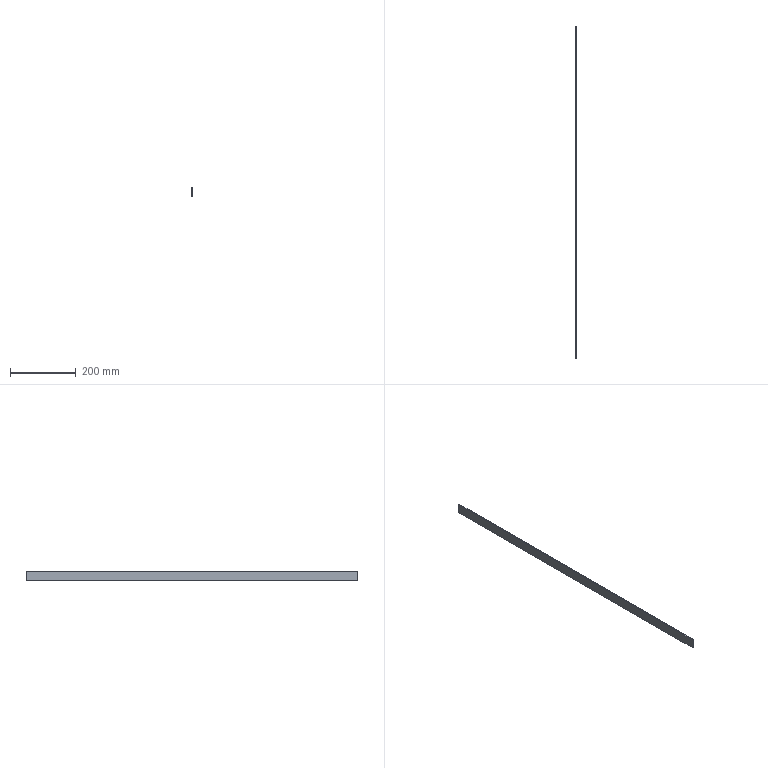Part | SolidWorks | 1 solid | 6 faces | box 3 x 1010 x 30 mm | volume 90900 mm3 | plane 6
STEP:
#1=CARTESIAN_POINT('',(0.,505.,15.));
#2=VERTEX_POINT('',#1);
#3=CARTESIAN_POINT('',(0.,-505.,15.));
#4=VERTEX_POINT('',#3);
#5=CARTESIAN_POINT('',(0.,-505.,15.));
#6=DIRECTION('',(0.,-1.,0.));
#7=VECTOR('',#6,1000.);
#8=LINE('',#5,#7);
#9=EDGE_CURVE('',#2,#4,#8,.T.);
#10=ORIENTED_EDGE('',*,*,#9,.F.);
#11=CARTESIAN_POINT('',(-3.,505.,15.));
#12=VERTEX_POINT('',#11);
#13=CARTESIAN_POINT('',(-3.,505.,15.));
#14=DIRECTION('',(1.,0.,0.));
#15=VECTOR('',#14,1000.);
#16=LINE('',#13,#15);
#17=EDGE_CURVE('',#12,#2,#16,.T.);
#18=ORIENTED_EDGE('',*,*,#17,.F.);
#19=CARTESIAN_POINT('',(-3.,-505.,15.));
#20=VERTEX_POINT('',#19);
#21=CARTESIAN_POINT('',(-3.,-505.,15.));
#22=DIRECTION('',(0.,-1.,0.));
#23=VECTOR('',#22,1000.);
#24=LINE('',#21,#23);
#25=EDGE_CURVE('',#12,#20,#24,.T.);
#26=ORIENTED_EDGE('',*,*,#25,.T.);
#27=CARTESIAN_POINT('',(-3.,-505.,15.));
#28=DIRECTION('',(1.,0.,0.));
#29=VECTOR('',#28,1000.);
#30=LINE('',#27,#29);
#31=EDGE_CURVE('',#20,#4,#30,.T.);
#32=ORIENTED_EDGE('',*,*,#31,.T.);
#33=EDGE_LOOP('',(#10,#18,#26,#32));
#34=FACE_OUTER_BOUND('',#33,.T.);
#35=CARTESIAN_POINT('',(-3.,-505.,15.));
#36=DIRECTION('',(0.,0.,1.));
#37=DIRECTION('',(1.,0.,0.));
#38=AXIS2_PLACEMENT_3D('',#35,#36,#37);
#39=PLANE('',#38);
#40=ADVANCED_FACE('',(#34),#39,.T.);
#41=CARTESIAN_POINT('',(0.,505.,-15.));
#42=VERTEX_POINT('',#41);
#43=CARTESIAN_POINT('',(0.,505.,-15.));
#44=DIRECTION('',(0.,0.,1.));
#45=VECTOR('',#44,1000.);
#46=LINE('',#43,#45);
#47=EDGE_CURVE('',#42,#2,#46,.T.);
#48=ORIENTED_EDGE('',*,*,#47,.F.);
#49=CARTESIAN_POINT('',(-3.,505.,-15.));
#50=VERTEX_POINT('',#49);
#51=CARTESIAN_POINT('',(-3.,505.,-15.));
#52=DIRECTION('',(1.,0.,0.));
#53=VECTOR('',#52,1000.);
#54=LINE('',#51,#53);
#55=EDGE_CURVE('',#50,#42,#54,.T.);
#56=ORIENTED_EDGE('',*,*,#55,.F.);
#57=CARTESIAN_POINT('',(-3.,505.,-15.));
#58=DIRECTION('',(0.,0.,1.));
#59=VECTOR('',#58,1000.);
#60=LINE('',#57,#59);
#61=EDGE_CURVE('',#50,#12,#60,.T.);
#62=ORIENTED_EDGE('',*,*,#61,.T.);
#63=ORIENTED_EDGE('',*,*,#17,.T.);
#64=EDGE_LOOP('',(#48,#56,#62,#63));
#65=FACE_OUTER_BOUND('',#64,.T.);
#66=CARTESIAN_POINT('',(-3.,505.,-15.));
#67=DIRECTION('',(0.,1.,0.));
#68=DIRECTION('',(0.,0.,1.));
#69=AXIS2_PLACEMENT_3D('',#66,#67,#68);
#70=PLANE('',#69);
#71=ADVANCED_FACE('',(#65),#70,.T.);
#72=CARTESIAN_POINT('',(0.,-505.,-15.));
#73=VERTEX_POINT('',#72);
#74=CARTESIAN_POINT('',(0.,-505.,-15.));
#75=DIRECTION('',(0.,1.,0.));
#76=VECTOR('',#75,1000.);
#77=LINE('',#74,#76);
#78=EDGE_CURVE('',#73,#42,#77,.T.);
#79=ORIENTED_EDGE('',*,*,#78,.F.);
#80=CARTESIAN_POINT('',(-3.,-505.,-15.));
#81=VERTEX_POINT('',#80);
#82=CARTESIAN_POINT('',(-3.,-505.,-15.));
#83=DIRECTION('',(1.,0.,0.));
#84=VECTOR('',#83,1000.);
#85=LINE('',#82,#84);
#86=EDGE_CURVE('',#81,#73,#85,.T.);
#87=ORIENTED_EDGE('',*,*,#86,.F.);
#88=CARTESIAN_POINT('',(-3.,-505.,-15.));
#89=DIRECTION('',(0.,1.,0.));
#90=VECTOR('',#89,1000.);
#91=LINE('',#88,#90);
#92=EDGE_CURVE('',#81,#50,#91,.T.);
#93=ORIENTED_EDGE('',*,*,#92,.T.);
#94=ORIENTED_EDGE('',*,*,#55,.T.);
#95=EDGE_LOOP('',(#79,#87,#93,#94));
#96=FACE_OUTER_BOUND('',#95,.T.);
#97=CARTESIAN_POINT('',(-3.,-505.,-15.));
#98=DIRECTION('',(0.,0.,-1.));
#99=DIRECTION('',(-1.,0.,0.));
#100=AXIS2_PLACEMENT_3D('',#97,#98,#99);
#101=PLANE('',#100);
#102=ADVANCED_FACE('',(#96),#101,.T.);
#103=CARTESIAN_POINT('',(0.,-505.,-15.));
#104=DIRECTION('',(0.,0.,-1.));
#105=VECTOR('',#104,1000.);
#106=LINE('',#103,#105);
#107=EDGE_CURVE('',#4,#73,#106,.T.);
#108=ORIENTED_EDGE('',*,*,#107,.F.);
#109=ORIENTED_EDGE('',*,*,#31,.F.);
#110=CARTESIAN_POINT('',(-3.,-505.,-15.));
#111=DIRECTION('',(0.,0.,-1.));
#112=VECTOR('',#111,1000.);
#113=LINE('',#110,#112);
#114=EDGE_CURVE('',#20,#81,#113,.T.);
#115=ORIENTED_EDGE('',*,*,#114,.T.);
#116=ORIENTED_EDGE('',*,*,#86,.T.);
#117=EDGE_LOOP('',(#108,#109,#115,#116));
#118=FACE_OUTER_BOUND('',#117,.T.);
#119=CARTESIAN_POINT('',(-3.,-505.,-15.));
#120=DIRECTION('',(0.,-1.,0.));
#121=DIRECTION('',(0.,0.,-1.));
#122=AXIS2_PLACEMENT_3D('',#119,#120,#121);
#123=PLANE('',#122);
#124=ADVANCED_FACE('',(#118),#123,.T.);
#125=ORIENTED_EDGE('',*,*,#25,.F.);
#126=ORIENTED_EDGE('',*,*,#61,.F.);
#127=ORIENTED_EDGE('',*,*,#92,.F.);
#128=ORIENTED_EDGE('',*,*,#114,.F.);
#129=EDGE_LOOP('',(#125,#126,#127,#128));
#130=FACE_OUTER_BOUND('',#129,.T.);
#131=CARTESIAN_POINT('',(-3.,0.,0.));
#132=DIRECTION('',(1.,0.,0.));
#133=DIRECTION('',(0.,0.,-1.));
#134=AXIS2_PLACEMENT_3D('',#131,#132,#133);
#135=PLANE('',#134);
#136=ADVANCED_FACE('',(#130),#135,.F.);
#137=ORIENTED_EDGE('',*,*,#9,.T.);
#138=ORIENTED_EDGE('',*,*,#107,.T.);
#139=ORIENTED_EDGE('',*,*,#78,.T.);
#140=ORIENTED_EDGE('',*,*,#47,.T.);
#141=EDGE_LOOP('',(#137,#138,#139,#140));
#142=FACE_OUTER_BOUND('',#141,.T.);
#143=CARTESIAN_POINT('',(0.,0.,0.));
#144=DIRECTION('',(1.,0.,0.));
#145=DIRECTION('',(0.,0.,-1.));
#146=AXIS2_PLACEMENT_3D('',#143,#144,#145);
#147=PLANE('',#146);
#148=ADVANCED_FACE('',(#142),#147,.T.);
#149=CLOSED_SHELL('',(#40,#71,#102,#124,#136,#148));
#150=MANIFOLD_SOLID_BREP('',#149);
#151=CARTESIAN_POINT('',(0.,0.,0.));
#152=DIRECTION('',(0.,0.,1.));
#153=DIRECTION('',(1.,0.,0.));
#154=AXIS2_PLACEMENT_3D('',#151,#152,#153);
#155=(LENGTH_UNIT()NAMED_UNIT(*)SI_UNIT(.MILLI.,.METRE.));
#156=UNCERTAINTY_MEASURE_WITH_UNIT(LENGTH_MEASURE(0.00001),#155,'','');
#157=(NAMED_UNIT(*)PLANE_ANGLE_UNIT()SI_UNIT($,.RADIAN.));
#158=(NAMED_UNIT(*)SI_UNIT($,.STERADIAN.)SOLID_ANGLE_UNIT());
#159=(GEOMETRIC_REPRESENTATION_CONTEXT(3)GLOBAL_UNCERTAINTY_ASSIGNED_CONTEXT((#156))GLOBAL_UNIT_ASSIGNED_CONTEXT((#155,#157,#158))REPRESENTATION_CONTEXT('',''));
#160=ADVANCED_BREP_SHAPE_REPRESENTATION('',(#150,#154),#159);